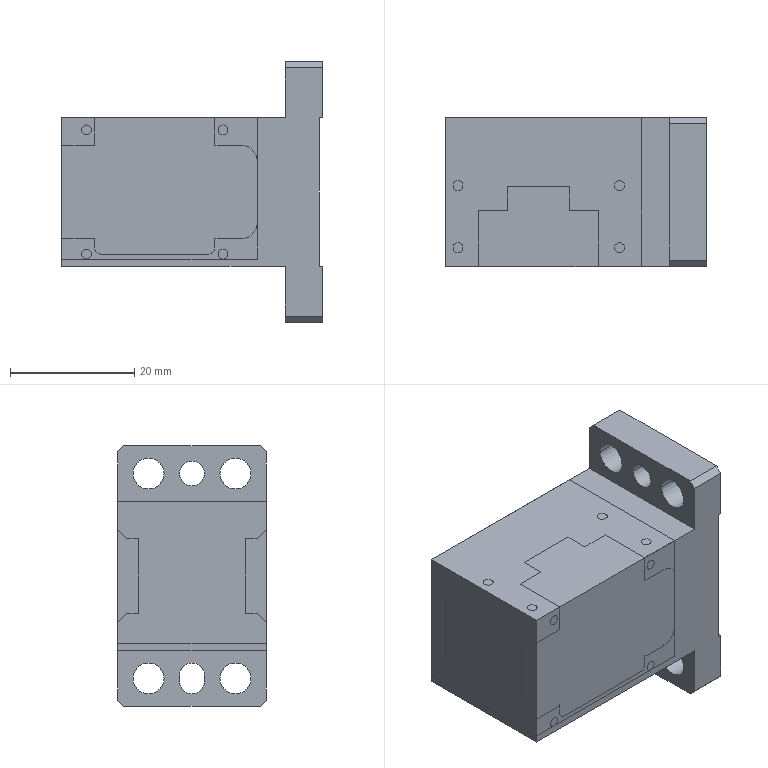NC program | NX | posted with a generic post | part box 42 x 24 x 42 mm
Lines 1 to 92 of 10692:
N10 G17 G21 G94 G90
(FLOOR_WALL_1_COPY_1 , TOOL : D10JING)
N12 T11 M6
N14 G54
N16 G17 G0 G90 X-18.5 Y-4.33 B0. C0. S5500 M3
N18 G43 Z30. H11
N20 Z1.333
N22 G94 G1 Z-0.167 F1000.
N24 X-12.5 Y-0.866
N26 G3 X-12. Y0. R1.
N28 G1 Y7. F1500.
N30 X12.
N32 Y-7.
N34 X-12.
N36 Y0.
N38 X-7.
N40 Y2.
N42 X7.
N44 Y-2.
N46 X-7.
N48 Y0.
N50 G3 X-7.5 Y0.866 R1.
N52 G1 Z1.333
N54 G0 X-18.5 Y-4.33 Z1.167
N56 G1 Z-0.333 F1000.
N58 X-12.5 Y-0.866
N60 G3 X-12. Y0. R1.
N62 G1 Y7. F1500.
N64 X12.
N66 Y-7.
N68 X-12.
N70 Y0.
N72 X-7.
N74 Y2.
N76 X7.
N78 Y-2.
N80 X-7.
N82 Y0.
N84 G3 X-7.5 Y0.866 R1.
N86 G1 Z1.167
N88 G0 X-18.5 Y-4.33 Z1.
N90 G1 Z-0.5 F1000.
N92 X-12.5 Y-0.866
N94 G3 X-12. Y0. R1.
N96 G1 Y7. F1500.
N98 X12.
N100 Y-7.
N102 X-12.
N104 Y0.
N106 X-7.
N108 Y2.
N110 X7.
N112 Y-2.
N114 X-7.
N116 Y0.
N118 G3 X-7.5 Y0.866 R1.
N120 G1 Z1.
N122 G0 Z30.
N124 M5
(DRILLING_1 , TOOL : ZXZ)
N126 T08 M6
N128 G54
N130 G17 G0 G90 X-7. Y16.5 B0. C0. S5000 M3
N132 G43 Z30. H8
N134 G94 G81 G98 Z-1. F250. R3.
N136 X0.
N138 X7.
N140 Y-16.5
N142 X-7.
N144 G80
N146 G0 X-7. Y-16.5 Z30.
N148 M5
(DRILLING_COPY_1 , TOOL : 5.0ZT)
N150 T14 M6
N152 G54
N154 G17 G0 G90 X-7. Y16.5 B0. C0. S2000 M3
N156 G43 Z30. H14
N158 G94 G83 G98 Z-8.852 F200. Q2. R3.
N160 X7.
N162 Y-16.5
N164 X-7.
N166 G80
N168 G0 X-7. Y-16.5 Z30.
N170 M5